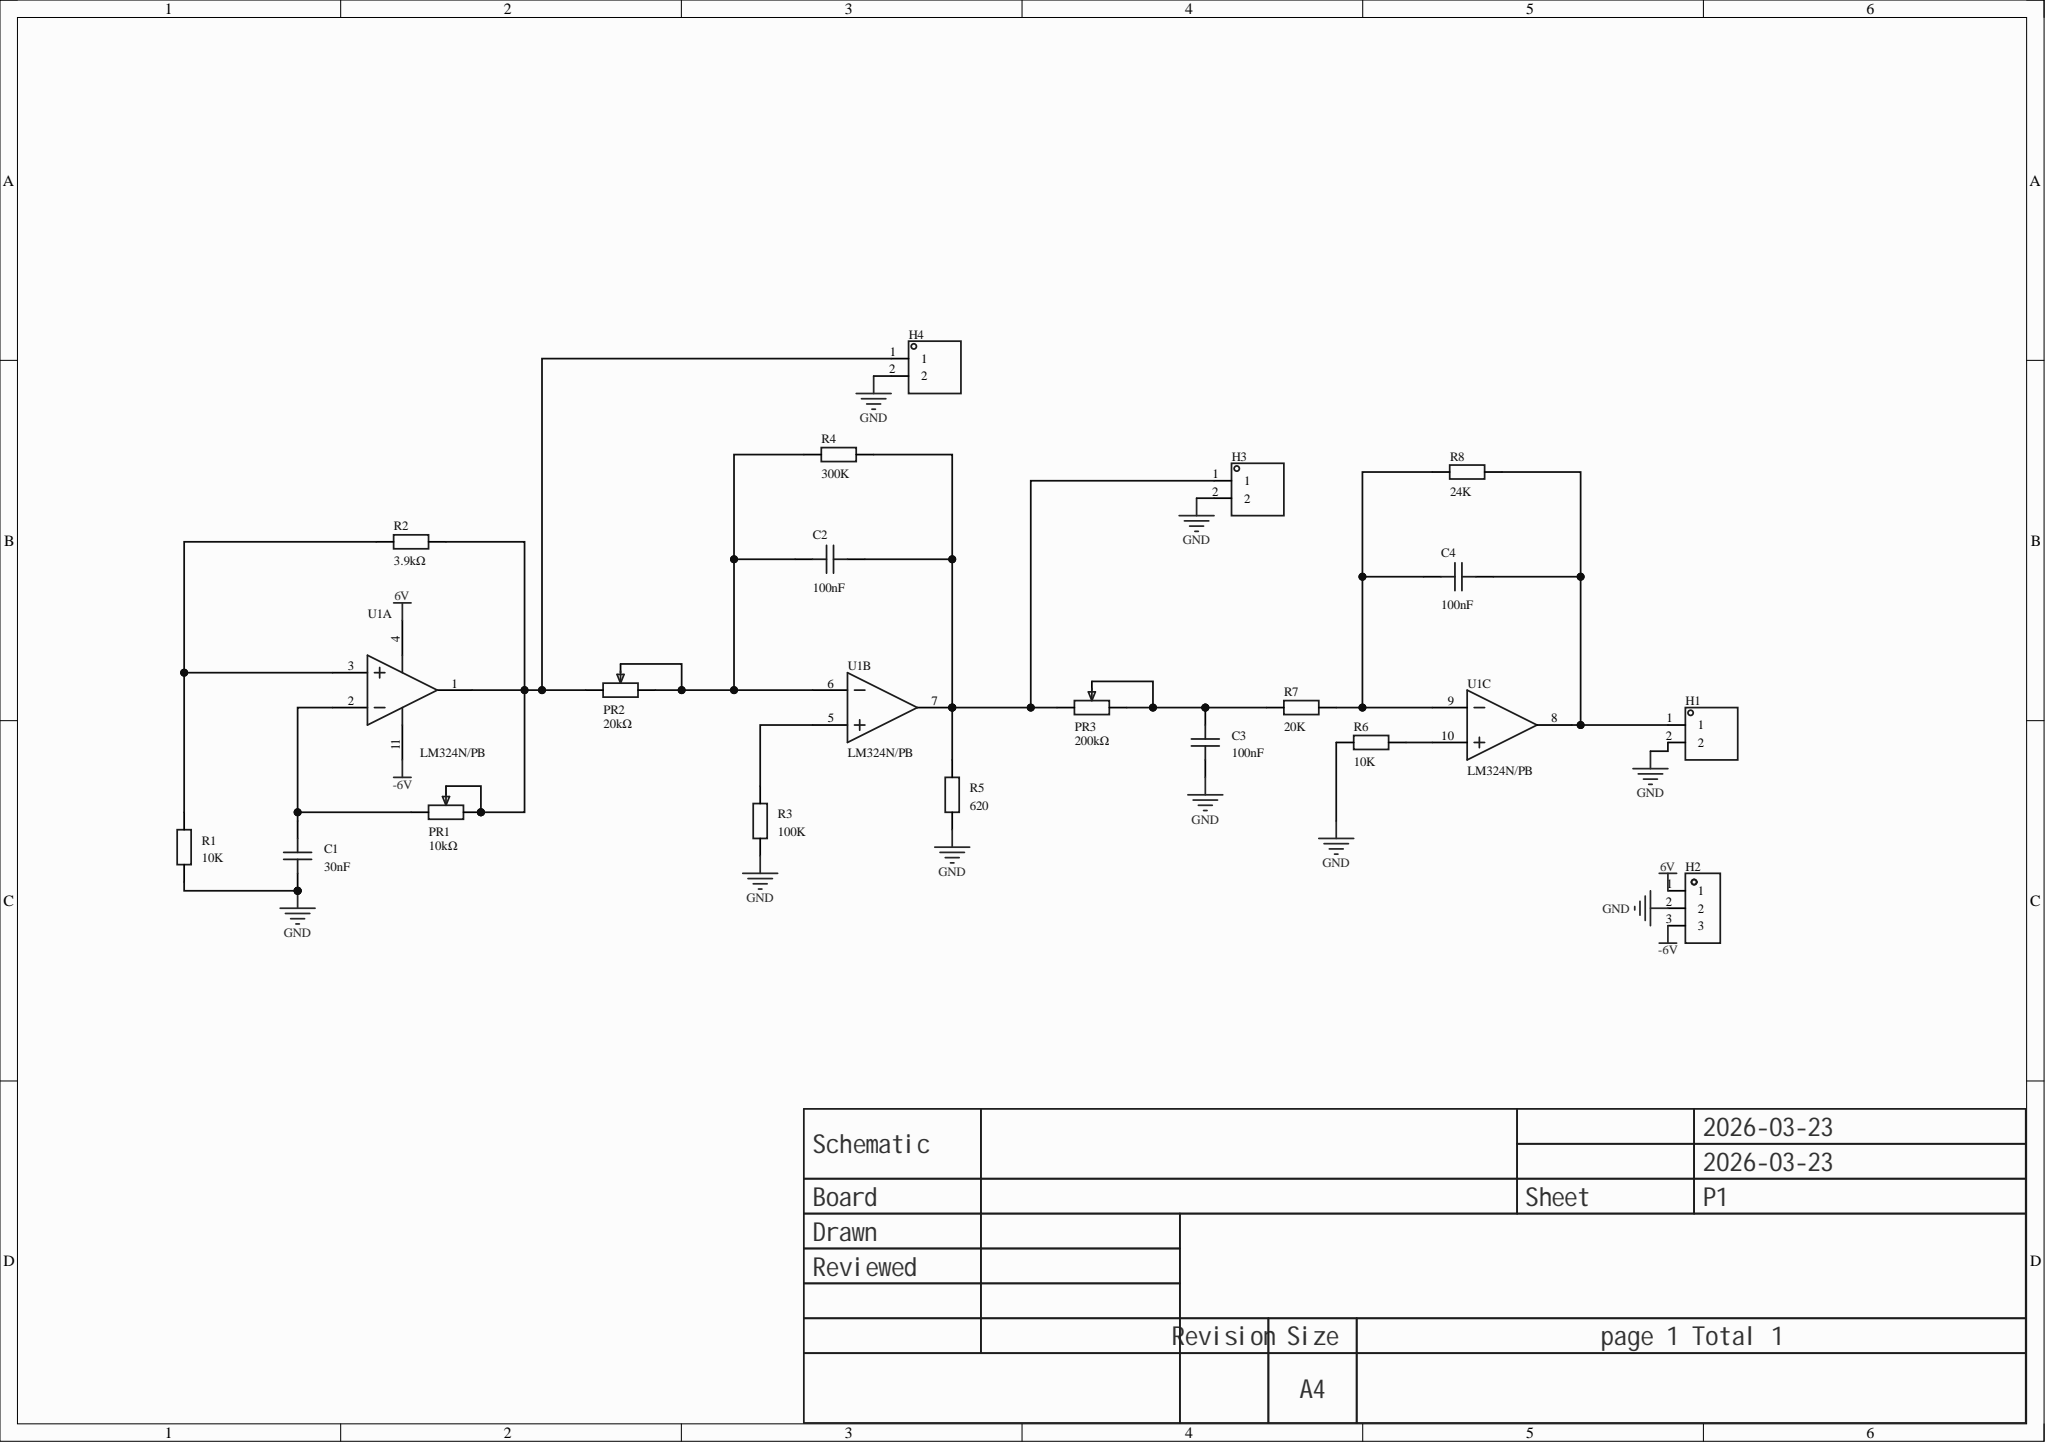Circuit board | Altium Designer | 20 parts | 13 nets
Bill of materials:
Comment,Description,Designator,Footprint,LibRef,Quantity
"30nF","","C1","C0603","CAP_0603","1"
"100nF","","C2, C3, C4","C0603","CAP_0603","3"
"","","H1, H3, H4","HDR-TH_2P-P2.54-V-M-1","HDR-M_2.54_1x2P","3"
"","","H2","HDR-TH_3P-P2.54-V-M","HDR-M_2.54_1x3P","1"
"10kΩ","","PR1","R_3296","R_3296","1"
"20kΩ","","PR2","R_3296","R_3296","1"
"200kΩ","","PR3","R_3296","R_3296","1"
"10K","","R1, R6","R0603","Res_0603","2"
"3.9kΩ","","R2","R0603","Res_0603","1"
"100K","","R3","R0603","Res_0603","1"
"300K","","R4","R0603","Res_0603","1"
"620","","R5","R0603","Res_0603","1"
"20K","","R7","R0603","Res_0603","1"
"24K","","R8","R0603","Res_0603","1"
"LM324N/PB","Amplifiers: quad; gain-bandwidth product (GBP): 1MHz; input bias current (Ib): 45nA;","U1","PDIP-14_L19.2-W6.6-P2.54-LS7.6-BL","LM324N/PB","1"
Netlist (Protel format):
[
C1
C0603
30nF



]
[
C2
C0603
100nF



]
[
C3
C0603
100nF



]
[
C4
C0603
100nF



]
[
H1
HDR-TH_2P-P2.54-V-M-1




]
[
H2
HDR-TH_3P-P2.54-V-M




]
[
H3
HDR-TH_2P-P2.54-V-M-1




]
[
H4
HDR-TH_2P-P2.54-V-M-1




]
[
PR1
R_3296
10kΩ



]
[
PR2
R_3296
20kΩ



]
[
PR3
R_3296
200kΩ



]
[
R1
R0603
10K



]
[
R2
R0603
3.9kΩ



]
[
R3
R0603
100K



]
[
R4
R0603
300K



]
[
R5
R0603
620



]
[
R6
R0603
10K



]
[
R7
R0603
20K



]
[
R8
R0603
24K



]
[
U1
PDIP-14_L19.2-W6.6-P2.54-LS7.6-BL
LM324N/PB



]
(
NetR6_2
R6-2
U1-10
)
(
NetR3_2
R3-2
U1-5
)
(
NetR1_2
R1-2
R2-2
U1-3
)
(
NetH4_1
H4-1
PR1-1
PR1-2
PR2-3
R2-1
U1-1
)
(
NetC4_2
C4-2
H1-1
R8-2
U1-8
)
(
NetC4_1
C4-1
R7-2
R8-1
U1-9
)
(
NetC3_2
C3-2
PR3-1
PR3-2
R7-1
)
(
NetC2_2
C2-2
H3-1
PR3-3
R4-2
R5-2
U1-7
)
(
NetC2_1
C2-1
PR2-1
PR2-2
R4-1
U1-6
)
(
NetC1_2
C1-2
PR1-3
U1-2
)
(
GND
C1-1
C3-1
H1-2
H2-2
H3-2
H4-2
R1-1
R3-1
R5-1
R6-1
)
(
-6V
H2-3
U1-11
)
(
6V
H2-1
U1-4
)